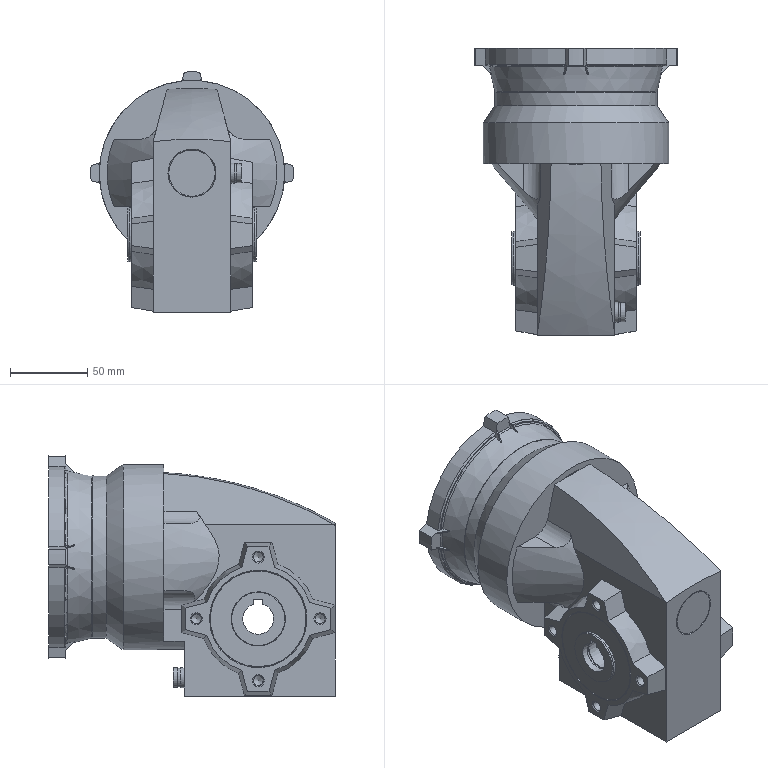Part | STEP file | 7 | 1 solid | 312 faces | box 131 x 185.7 x 155.5 mm | volume 1497643 mm3 | plane 157 | cylinder 76 | cone 56 | torus 22 | spline 1 | commonest cylinder face diameters 6.4 x10 6.39 x8 7 x8 4.79 x4 4.8 x4 20 x4